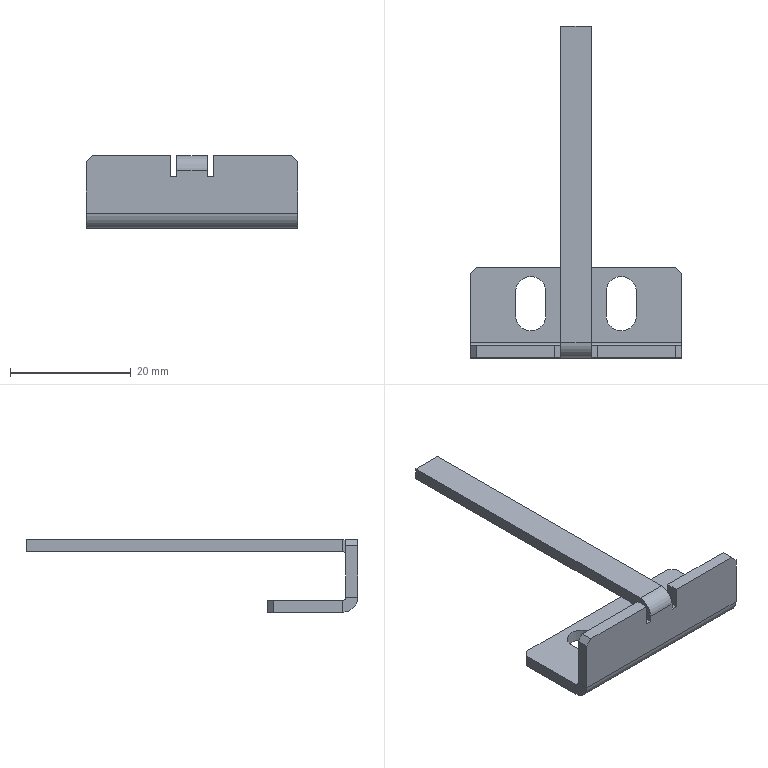Part | SolidWorks | features EdgeFlange 2, Chamfer 1, FlatPattern 1, HoleWzd 1, SMBaseFlange 1, SheetMetal 1 | 1 solid | 42 faces | box 35 x 55 x 12 mm | volume 2052 mm3 | plane 34 | cylinder 8 | commonest cylinder face diameters 5 x6 1 x2
STEP:
#1=CARTESIAN_POINT('',(-16.5,-7.5,10.));
#2=VERTEX_POINT('',#1);
#3=CARTESIAN_POINT('',(-3.5,-7.5,10.));
#4=VERTEX_POINT('',#3);
#5=CARTESIAN_POINT('',(17.5,-7.5,10.));
#6=DIRECTION('',(1.,0.,0.));
#7=VECTOR('',#6,1000.);
#8=LINE('',#5,#7);
#9=EDGE_CURVE('',#2,#4,#8,.T.);
#10=ORIENTED_EDGE('',*,*,#9,.F.);
#11=CARTESIAN_POINT('',(-17.5,-7.5,9.));
#12=VERTEX_POINT('',#11);
#13=CARTESIAN_POINT('',(-13.25,-7.5,13.25));
#14=DIRECTION('',(-0.7071,0.,-0.7071));
#15=VECTOR('',#14,1000.);
#16=LINE('',#13,#15);
#17=EDGE_CURVE('',#2,#12,#16,.T.);
#18=ORIENTED_EDGE('',*,*,#17,.T.);
#19=CARTESIAN_POINT('',(-17.5,-7.5,0.5));
#20=VERTEX_POINT('',#19);
#21=CARTESIAN_POINT('',(-17.5,-7.5,10.));
#22=DIRECTION('',(0.,0.,1.));
#23=VECTOR('',#22,1000.);
#24=LINE('',#21,#23);
#25=EDGE_CURVE('',#20,#12,#24,.T.);
#26=ORIENTED_EDGE('',*,*,#25,.F.);
#27=CARTESIAN_POINT('',(17.5,-7.5,0.5));
#28=VERTEX_POINT('',#27);
#29=CARTESIAN_POINT('',(0.,-7.5,0.5));
#30=DIRECTION('',(1.,0.,0.));
#31=VECTOR('',#30,1000.);
#32=LINE('',#29,#31);
#33=EDGE_CURVE('',#20,#28,#32,.T.);
#34=ORIENTED_EDGE('',*,*,#33,.T.);
#35=CARTESIAN_POINT('',(17.5,-7.5,9.));
#36=VERTEX_POINT('',#35);
#37=CARTESIAN_POINT('',(17.5,-7.5,0.));
#38=DIRECTION('',(0.,0.,-1.));
#39=VECTOR('',#38,1000.);
#40=LINE('',#37,#39);
#41=EDGE_CURVE('',#36,#28,#40,.T.);
#42=ORIENTED_EDGE('',*,*,#41,.F.);
#43=CARTESIAN_POINT('',(16.5,-7.5,10.));
#44=VERTEX_POINT('',#43);
#45=CARTESIAN_POINT('',(13.25,-7.5,13.25));
#46=DIRECTION('',(-0.7071,0.,0.7071));
#47=VECTOR('',#46,1000.);
#48=LINE('',#45,#47);
#49=EDGE_CURVE('',#36,#44,#48,.T.);
#50=ORIENTED_EDGE('',*,*,#49,.T.);
#51=CARTESIAN_POINT('',(3.5,-7.5,10.));
#52=VERTEX_POINT('',#51);
#53=CARTESIAN_POINT('',(17.5,-7.5,10.));
#54=DIRECTION('',(1.,0.,0.));
#55=VECTOR('',#54,1000.);
#56=LINE('',#53,#55);
#57=EDGE_CURVE('',#52,#44,#56,.T.);
#58=ORIENTED_EDGE('',*,*,#57,.F.);
#59=CARTESIAN_POINT('',(3.5,-7.5,6.5));
#60=VERTEX_POINT('',#59);
#61=CARTESIAN_POINT('',(3.5,-7.5,0.));
#62=DIRECTION('',(0.,0.,-1.));
#63=VECTOR('',#62,1000.);
#64=LINE('',#61,#63);
#65=EDGE_CURVE('',#52,#60,#64,.T.);
#66=ORIENTED_EDGE('',*,*,#65,.T.);
#67=CARTESIAN_POINT('',(2.5,-7.5,6.5));
#68=VERTEX_POINT('',#67);
#69=CARTESIAN_POINT('',(0.,-7.5,6.5));
#70=DIRECTION('',(-1.,0.,0.));
#71=VECTOR('',#70,1000.);
#72=LINE('',#69,#71);
#73=EDGE_CURVE('',#60,#68,#72,.T.);
#74=ORIENTED_EDGE('',*,*,#73,.T.);
#75=CARTESIAN_POINT('',(2.5,-7.5,7.5));
#76=VERTEX_POINT('',#75);
#77=CARTESIAN_POINT('',(2.5,-7.5,0.));
#78=DIRECTION('',(0.,0.,1.));
#79=VECTOR('',#78,1000.);
#80=LINE('',#77,#79);
#81=EDGE_CURVE('',#68,#76,#80,.T.);
#82=ORIENTED_EDGE('',*,*,#81,.T.);
#83=CARTESIAN_POINT('',(-2.5,-7.5,7.5));
#84=VERTEX_POINT('',#83);
#85=CARTESIAN_POINT('',(2.5,-7.5,7.5));
#86=DIRECTION('',(-1.,0.,0.));
#87=VECTOR('',#86,1000.);
#88=LINE('',#85,#87);
#89=EDGE_CURVE('',#76,#84,#88,.T.);
#90=ORIENTED_EDGE('',*,*,#89,.T.);
#91=CARTESIAN_POINT('',(-2.5,-7.5,6.5));
#92=VERTEX_POINT('',#91);
#93=CARTESIAN_POINT('',(-2.5,-7.5,0.));
#94=DIRECTION('',(0.,0.,-1.));
#95=VECTOR('',#94,1000.);
#96=LINE('',#93,#95);
#97=EDGE_CURVE('',#84,#92,#96,.T.);
#98=ORIENTED_EDGE('',*,*,#97,.T.);
#99=CARTESIAN_POINT('',(-3.5,-7.5,6.5));
#100=VERTEX_POINT('',#99);
#101=CARTESIAN_POINT('',(0.,-7.5,6.5));
#102=DIRECTION('',(-1.,0.,0.));
#103=VECTOR('',#102,1000.);
#104=LINE('',#101,#103);
#105=EDGE_CURVE('',#92,#100,#104,.T.);
#106=ORIENTED_EDGE('',*,*,#105,.T.);
#107=CARTESIAN_POINT('',(-3.5,-7.5,0.));
#108=DIRECTION('',(0.,0.,1.));
#109=VECTOR('',#108,1000.);
#110=LINE('',#107,#109);
#111=EDGE_CURVE('',#100,#4,#110,.T.);
#112=ORIENTED_EDGE('',*,*,#111,.T.);
#113=EDGE_LOOP('',(#10,#18,#26,#34,#42,#50,#58,#66,#74,#82,#90,#98,#106,#112));
#114=FACE_OUTER_BOUND('',#113,.T.);
#115=CARTESIAN_POINT('',(0.,-7.5,0.));
#116=DIRECTION('',(0.,-1.,0.));
#117=DIRECTION('',(0.,0.,-1.));
#118=AXIS2_PLACEMENT_3D('',#115,#116,#117);
#119=PLANE('',#118);
#120=ADVANCED_FACE('',(#114),#119,.T.);
#121=CARTESIAN_POINT('',(-17.5,-5.5,0.5));
#122=VERTEX_POINT('',#121);
#123=CARTESIAN_POINT('',(-17.5,-5.5,9.));
#124=VERTEX_POINT('',#123);
#125=CARTESIAN_POINT('',(-17.5,-5.5,0.));
#126=DIRECTION('',(0.,0.,1.));
#127=VECTOR('',#126,1000.);
#128=LINE('',#125,#127);
#129=EDGE_CURVE('',#122,#124,#128,.T.);
#130=ORIENTED_EDGE('',*,*,#129,.T.);
#131=CARTESIAN_POINT('',(-16.5,-5.5,10.));
#132=VERTEX_POINT('',#131);
#133=CARTESIAN_POINT('',(-17.5,-5.5,9.));
#134=DIRECTION('',(0.7071,0.,0.7071));
#135=VECTOR('',#134,1000.);
#136=LINE('',#133,#135);
#137=EDGE_CURVE('',#124,#132,#136,.T.);
#138=ORIENTED_EDGE('',*,*,#137,.T.);
#139=CARTESIAN_POINT('',(-3.5,-5.5,10.));
#140=VERTEX_POINT('',#139);
#141=CARTESIAN_POINT('',(0.,-5.5,10.));
#142=DIRECTION('',(1.,0.,0.));
#143=VECTOR('',#142,1000.);
#144=LINE('',#141,#143);
#145=EDGE_CURVE('',#132,#140,#144,.T.);
#146=ORIENTED_EDGE('',*,*,#145,.T.);
#147=CARTESIAN_POINT('',(-3.5,-5.5,6.5));
#148=VERTEX_POINT('',#147);
#149=CARTESIAN_POINT('',(-3.5,-5.5,6.5));
#150=DIRECTION('',(0.,0.,1.));
#151=VECTOR('',#150,1000.);
#152=LINE('',#149,#151);
#153=EDGE_CURVE('',#148,#140,#152,.T.);
#154=ORIENTED_EDGE('',*,*,#153,.F.);
#155=CARTESIAN_POINT('',(-2.5,-5.5,6.5));
#156=VERTEX_POINT('',#155);
#157=CARTESIAN_POINT('',(-2.5,-5.5,6.5));
#158=DIRECTION('',(-1.,0.,0.));
#159=VECTOR('',#158,1000.);
#160=LINE('',#157,#159);
#161=EDGE_CURVE('',#156,#148,#160,.T.);
#162=ORIENTED_EDGE('',*,*,#161,.F.);
#163=CARTESIAN_POINT('',(-2.5,-5.5,7.5));
#164=VERTEX_POINT('',#163);
#165=CARTESIAN_POINT('',(-2.5,-5.5,7.5));
#166=DIRECTION('',(0.,0.,-1.));
#167=VECTOR('',#166,1000.);
#168=LINE('',#165,#167);
#169=EDGE_CURVE('',#164,#156,#168,.T.);
#170=ORIENTED_EDGE('',*,*,#169,.F.);
#171=CARTESIAN_POINT('',(2.5,-5.5,7.5));
#172=VERTEX_POINT('',#171);
#173=CARTESIAN_POINT('',(2.5,-5.5,7.5));
#174=DIRECTION('',(-1.,0.,0.));
#175=VECTOR('',#174,1000.);
#176=LINE('',#173,#175);
#177=EDGE_CURVE('',#172,#164,#176,.T.);
#178=ORIENTED_EDGE('',*,*,#177,.F.);
#179=CARTESIAN_POINT('',(2.5,-5.5,6.5));
#180=VERTEX_POINT('',#179);
#181=CARTESIAN_POINT('',(2.5,-5.5,6.5));
#182=DIRECTION('',(0.,0.,1.));
#183=VECTOR('',#182,1000.);
#184=LINE('',#181,#183);
#185=EDGE_CURVE('',#180,#172,#184,.T.);
#186=ORIENTED_EDGE('',*,*,#185,.F.);
#187=CARTESIAN_POINT('',(3.5,-5.5,6.5));
#188=VERTEX_POINT('',#187);
#189=CARTESIAN_POINT('',(3.5,-5.5,6.5));
#190=DIRECTION('',(-1.,0.,0.));
#191=VECTOR('',#190,1000.);
#192=LINE('',#189,#191);
#193=EDGE_CURVE('',#188,#180,#192,.T.);
#194=ORIENTED_EDGE('',*,*,#193,.F.);
#195=CARTESIAN_POINT('',(3.5,-5.5,10.));
#196=VERTEX_POINT('',#195);
#197=CARTESIAN_POINT('',(3.5,-5.5,10.));
#198=DIRECTION('',(0.,0.,-1.));
#199=VECTOR('',#198,1000.);
#200=LINE('',#197,#199);
#201=EDGE_CURVE('',#196,#188,#200,.T.);
#202=ORIENTED_EDGE('',*,*,#201,.F.);
#203=CARTESIAN_POINT('',(16.5,-5.5,10.));
#204=VERTEX_POINT('',#203);
#205=CARTESIAN_POINT('',(0.,-5.5,10.));
#206=DIRECTION('',(1.,0.,0.));
#207=VECTOR('',#206,1000.);
#208=LINE('',#205,#207);
#209=EDGE_CURVE('',#196,#204,#208,.T.);
#210=ORIENTED_EDGE('',*,*,#209,.T.);
#211=CARTESIAN_POINT('',(17.5,-5.5,9.));
#212=VERTEX_POINT('',#211);
#213=CARTESIAN_POINT('',(16.5,-5.5,10.));
#214=DIRECTION('',(0.7071,0.,-0.7071));
#215=VECTOR('',#214,1000.);
#216=LINE('',#213,#215);
#217=EDGE_CURVE('',#204,#212,#216,.T.);
#218=ORIENTED_EDGE('',*,*,#217,.T.);
#219=CARTESIAN_POINT('',(17.5,-5.5,0.5));
#220=VERTEX_POINT('',#219);
#221=CARTESIAN_POINT('',(17.5,-5.5,0.));
#222=DIRECTION('',(0.,0.,-1.));
#223=VECTOR('',#222,1000.);
#224=LINE('',#221,#223);
#225=EDGE_CURVE('',#212,#220,#224,.T.);
#226=ORIENTED_EDGE('',*,*,#225,.T.);
#227=CARTESIAN_POINT('',(-17.5,-5.5,0.5));
#228=DIRECTION('',(1.,0.,0.));
#229=VECTOR('',#228,1000.);
#230=LINE('',#227,#229);
#231=EDGE_CURVE('',#122,#220,#230,.T.);
#232=ORIENTED_EDGE('',*,*,#231,.F.);
#233=EDGE_LOOP('',(#130,#138,#146,#154,#162,#170,#178,#186,#194,#202,#210,#218,#226,#232));
#234=FACE_OUTER_BOUND('',#233,.T.);
#235=CARTESIAN_POINT('',(0.,-5.5,0.));
#236=DIRECTION('',(0.,-1.,0.));
#237=DIRECTION('',(0.,0.,-1.));
#238=AXIS2_PLACEMENT_3D('',#235,#236,#237);
#239=PLANE('',#238);
#240=ADVANCED_FACE('',(#234),#239,.F.);
#241=ORIENTED_EDGE('',*,*,#57,.T.);
#242=CARTESIAN_POINT('',(16.5,-7.5,10.));
#243=DIRECTION('',(0.,1.,0.));
#244=VECTOR('',#243,1000.);
#245=LINE('',#242,#244);
#246=EDGE_CURVE('',#44,#204,#245,.T.);
#247=ORIENTED_EDGE('',*,*,#246,.T.);
#248=ORIENTED_EDGE('',*,*,#209,.F.);
#249=CARTESIAN_POINT('',(3.5,-5.5,10.));
#250=DIRECTION('',(0.,-1.,0.));
#251=VECTOR('',#250,1000.);
#252=LINE('',#249,#251);
#253=EDGE_CURVE('',#196,#52,#252,.T.);
#254=ORIENTED_EDGE('',*,*,#253,.T.);
#255=EDGE_LOOP('',(#241,#247,#248,#254));
#256=FACE_OUTER_BOUND('',#255,.T.);
#257=CARTESIAN_POINT('',(17.5,-7.5,10.));
#258=DIRECTION('',(0.,0.,1.));
#259=DIRECTION('',(0.,-1.,0.));
#260=AXIS2_PLACEMENT_3D('',#257,#258,#259);
#261=PLANE('',#260);
#262=ADVANCED_FACE('',(#256),#261,.T.);
#263=ORIENTED_EDGE('',*,*,#145,.F.);
#264=CARTESIAN_POINT('',(-16.5,-7.5,10.));
#265=DIRECTION('',(0.,-1.,0.));
#266=VECTOR('',#265,1000.);
#267=LINE('',#264,#266);
#268=EDGE_CURVE('',#132,#2,#267,.T.);
#269=ORIENTED_EDGE('',*,*,#268,.T.);
#270=ORIENTED_EDGE('',*,*,#9,.T.);
#271=CARTESIAN_POINT('',(-3.5,-5.5,10.));
#272=DIRECTION('',(0.,-1.,0.));
#273=VECTOR('',#272,1000.);
#274=LINE('',#271,#273);
#275=EDGE_CURVE('',#140,#4,#274,.T.);
#276=ORIENTED_EDGE('',*,*,#275,.F.);
#277=EDGE_LOOP('',(#263,#269,#270,#276));
#278=FACE_OUTER_BOUND('',#277,.T.);
#279=CARTESIAN_POINT('',(17.5,-7.5,10.));
#280=DIRECTION('',(0.,0.,1.));
#281=DIRECTION('',(0.,-1.,0.));
#282=AXIS2_PLACEMENT_3D('',#279,#280,#281);
#283=PLANE('',#282);
#284=ADVANCED_FACE('',(#278),#283,.T.);
#285=CARTESIAN_POINT('',(17.5,-5.,-2.));
#286=VERTEX_POINT('',#285);
#287=CARTESIAN_POINT('',(17.5,6.5,-2.));
#288=VERTEX_POINT('',#287);
#289=CARTESIAN_POINT('',(17.5,7.5,-2.));
#290=DIRECTION('',(0.,1.,0.));
#291=VECTOR('',#290,1000.);
#292=LINE('',#289,#291);
#293=EDGE_CURVE('',#286,#288,#292,.T.);
#294=ORIENTED_EDGE('',*,*,#293,.T.);
#295=CARTESIAN_POINT('',(17.5,6.5,0.));
#296=VERTEX_POINT('',#295);
#297=CARTESIAN_POINT('',(17.5,6.5,-2.));
#298=DIRECTION('',(0.,0.,1.));
#299=VECTOR('',#298,1000.);
#300=LINE('',#297,#299);
#301=EDGE_CURVE('',#288,#296,#300,.T.);
#302=ORIENTED_EDGE('',*,*,#301,.T.);
#303=CARTESIAN_POINT('',(17.5,-5.,0.));
#304=VERTEX_POINT('',#303);
#305=CARTESIAN_POINT('',(17.5,7.5,0.));
#306=DIRECTION('',(0.,1.,0.));
#307=VECTOR('',#306,1000.);
#308=LINE('',#305,#307);
#309=EDGE_CURVE('',#304,#296,#308,.T.);
#310=ORIENTED_EDGE('',*,*,#309,.F.);
#311=CARTESIAN_POINT('',(17.5,-5.,0.));
#312=DIRECTION('',(0.,0.,-1.));
#313=VECTOR('',#312,1000.);
#314=LINE('',#311,#313);
#315=EDGE_CURVE('',#304,#286,#314,.T.);
#316=ORIENTED_EDGE('',*,*,#315,.T.);
#317=EDGE_LOOP('',(#294,#302,#310,#316));
#318=FACE_OUTER_BOUND('',#317,.T.);
#319=CARTESIAN_POINT('',(17.5,7.5,-2.));
#320=DIRECTION('',(1.,0.,0.));
#321=DIRECTION('',(0.,0.,-1.));
#322=AXIS2_PLACEMENT_3D('',#319,#320,#321);
#323=PLANE('',#322);
#324=ADVANCED_FACE('',(#318),#323,.T.);
#325=CARTESIAN_POINT('',(-10.,-0.5,-2.));
#326=VERTEX_POINT('',#325);
#327=CARTESIAN_POINT('',(-10.,3.5,-2.));
#328=VERTEX_POINT('',#327);
#329=CARTESIAN_POINT('',(-10.,-0.5,-2.));
#330=DIRECTION('',(0.,1.,0.));
#331=VECTOR('',#330,1000.);
#332=LINE('',#329,#331);
#333=EDGE_CURVE('',#326,#328,#332,.T.);
#334=ORIENTED_EDGE('',*,*,#333,.F.);
#335=CARTESIAN_POINT('',(-5.,-0.5,-2.));
#336=VERTEX_POINT('',#335);
#337=CARTESIAN_POINT('',(-7.5,-0.5,-2.));
#338=DIRECTION('',(0.,0.,1.));
#339=DIRECTION('',(1.,0.,0.));
#340=AXIS2_PLACEMENT_3D('',#337,#338,#339);
#341=CIRCLE('',#340,2.5);
#342=EDGE_CURVE('',#326,#336,#341,.T.);
#343=ORIENTED_EDGE('',*,*,#342,.T.);
#344=CARTESIAN_POINT('',(-5.,3.5,-2.));
#345=VERTEX_POINT('',#344);
#346=CARTESIAN_POINT('',(-5.,-0.5,-2.));
#347=DIRECTION('',(0.,1.,0.));
#348=VECTOR('',#347,1000.);
#349=LINE('',#346,#348);
#350=EDGE_CURVE('',#336,#345,#349,.T.);
#351=ORIENTED_EDGE('',*,*,#350,.T.);
#352=CARTESIAN_POINT('',(-7.5,3.5,-2.));
#353=DIRECTION('',(0.,0.,1.));
#354=DIRECTION('',(1.,0.,0.));
#355=AXIS2_PLACEMENT_3D('',#352,#353,#354);
#356=CIRCLE('',#355,2.5);
#357=EDGE_CURVE('',#345,#328,#356,.T.);
#358=ORIENTED_EDGE('',*,*,#357,.T.);
#359=EDGE_LOOP('',(#334,#343,#351,#358));
#360=FACE_BOUND('',#359,.T.);
#361=CARTESIAN_POINT('',(5.,-0.5,-2.));
#362=VERTEX_POINT('',#361);
#363=CARTESIAN_POINT('',(5.,3.5,-2.));
#364=VERTEX_POINT('',#363);
#365=CARTESIAN_POINT('',(5.,-0.5,-2.));
#366=DIRECTION('',(0.,1.,0.));
#367=VECTOR('',#366,1000.);
#368=LINE('',#365,#367);
#369=EDGE_CURVE('',#362,#364,#368,.T.);
#370=ORIENTED_EDGE('',*,*,#369,.F.);
#371=CARTESIAN_POINT('',(10.,-0.5,-2.));
#372=VERTEX_POINT('',#371);
#373=CARTESIAN_POINT('',(7.5,-0.5,-2.));
#374=DIRECTION('',(0.,0.,1.));
#375=DIRECTION('',(1.,0.,0.));
#376=AXIS2_PLACEMENT_3D('',#373,#374,#375);
#377=CIRCLE('',#376,2.5);
#378=EDGE_CURVE('',#362,#372,#377,.T.);
#379=ORIENTED_EDGE('',*,*,#378,.T.);
#380=CARTESIAN_POINT('',(10.,3.5,-2.));
#381=VERTEX_POINT('',#380);
#382=CARTESIAN_POINT('',(10.,-0.5,-2.));
#383=DIRECTION('',(0.,1.,0.));
#384=VECTOR('',#383,1000.);
#385=LINE('',#382,#384);
#386=EDGE_CURVE('',#372,#381,#385,.T.);
#387=ORIENTED_EDGE('',*,*,#386,.T.);
#388=CARTESIAN_POINT('',(7.5,3.5,-2.));
#389=DIRECTION('',(0.,0.,1.));
#390=DIRECTION('',(1.,0.,0.));
#391=AXIS2_PLACEMENT_3D('',#388,#389,#390);
#392=CIRCLE('',#391,2.5);
#393=EDGE_CURVE('',#381,#364,#392,.T.);
#394=ORIENTED_EDGE('',*,*,#393,.T.);
#395=EDGE_LOOP('',(#370,#379,#387,#394));
#396=FACE_BOUND('',#395,.T.);
#397=CARTESIAN_POINT('',(16.5,7.5,-2.));
#398=VERTEX_POINT('',#397);
#399=CARTESIAN_POINT('',(-16.5,7.5,-2.));
#400=VERTEX_POINT('',#399);
#401=CARTESIAN_POINT('',(-17.5,7.5,-2.));
#402=DIRECTION('',(-1.,0.,0.));
#403=VECTOR('',#402,1000.);
#404=LINE('',#401,#403);
#405=EDGE_CURVE('',#398,#400,#404,.T.);
#406=ORIENTED_EDGE('',*,*,#405,.F.);
#407=CARTESIAN_POINT('',(17.5,6.5,-2.));
#408=DIRECTION('',(0.7071,-0.7071,0.));
#409=VECTOR('',#408,1000.);
#410=LINE('',#407,#409);
#411=EDGE_CURVE('',#398,#288,#410,.T.);
#412=ORIENTED_EDGE('',*,*,#411,.T.);
#413=ORIENTED_EDGE('',*,*,#293,.F.);
#414=CARTESIAN_POINT('',(-17.5,-5.,-2.));
#415=VERTEX_POINT('',#414);
#416=CARTESIAN_POINT('',(17.5,-5.,-2.));
#417=DIRECTION('',(-1.,0.,0.));
#418=VECTOR('',#417,1000.);
#419=LINE('',#416,#418);
#420=EDGE_CURVE('',#286,#415,#419,.T.);
#421=ORIENTED_EDGE('',*,*,#420,.T.);
#422=CARTESIAN_POINT('',(-17.5,6.5,-2.));
#423=VERTEX_POINT('',#422);
#424=CARTESIAN_POINT('',(-17.5,7.5,-2.));
#425=DIRECTION('',(0.,-1.,0.));
#426=VECTOR('',#425,1000.);
#427=LINE('',#424,#426);
#428=EDGE_CURVE('',#423,#415,#427,.T.);
#429=ORIENTED_EDGE('',*,*,#428,.F.);
#430=CARTESIAN_POINT('',(-16.5,7.5,-2.));
#431=DIRECTION('',(0.7071,0.7071,0.));
#432=VECTOR('',#431,1000.);
#433=LINE('',#430,#432);
#434=EDGE_CURVE('',#423,#400,#433,.T.);
#435=ORIENTED_EDGE('',*,*,#434,.T.);
#436=EDGE_LOOP('',(#406,#412,#413,#421,#429,#435));
#437=FACE_OUTER_BOUND('',#436,.T.);
#438=CARTESIAN_POINT('',(0.,0.,-2.));
#439=DIRECTION('',(0.,0.,1.));
#440=DIRECTION('',(1.,0.,0.));
#441=AXIS2_PLACEMENT_3D('',#438,#439,#440);
#442=PLANE('',#441);
#443=ADVANCED_FACE('',(#360,#396,#437),#442,.F.);
#444=CARTESIAN_POINT('',(-5.,-0.5,0.));
#445=VERTEX_POINT('',#444);
#446=CARTESIAN_POINT('',(-5.,3.5,0.));
#447=VERTEX_POINT('',#446);
#448=CARTESIAN_POINT('',(-5.,-0.5,0.));
#449=DIRECTION('',(0.,1.,0.));
#450=VECTOR('',#449,1000.);
#451=LINE('',#448,#450);
#452=EDGE_CURVE('',#445,#447,#451,.T.);
#453=ORIENTED_EDGE('',*,*,#452,.F.);
#454=CARTESIAN_POINT('',(-10.,-0.5,0.));
#455=VERTEX_POINT('',#454);
#456=CARTESIAN_POINT('',(-7.5,-0.5,0.));
#457=DIRECTION('',(0.,0.,1.));
#458=DIRECTION('',(1.,0.,0.));
#459=AXIS2_PLACEMENT_3D('',#456,#457,#458);
#460=CIRCLE('',#459,2.5);
#461=EDGE_CURVE('',#455,#445,#460,.T.);
#462=ORIENTED_EDGE('',*,*,#461,.F.);
#463=CARTESIAN_POINT('',(-10.,3.5,0.));
#464=VERTEX_POINT('',#463);
#465=CARTESIAN_POINT('',(-10.,-0.5,0.));
#466=DIRECTION('',(0.,1.,0.));
#467=VECTOR('',#466,1000.);
#468=LINE('',#465,#467);
#469=EDGE_CURVE('',#455,#464,#468,.T.);
#470=ORIENTED_EDGE('',*,*,#469,.T.);
#471=CARTESIAN_POINT('',(-7.5,3.5,0.));
#472=DIRECTION('',(0.,0.,1.));
#473=DIRECTION('',(1.,0.,0.));
#474=AXIS2_PLACEMENT_3D('',#471,#472,#473);
#475=CIRCLE('',#474,2.5);
#476=EDGE_CURVE('',#447,#464,#475,.T.);
#477=ORIENTED_EDGE('',*,*,#476,.F.);
#478=EDGE_LOOP('',(#453,#462,#470,#477));
#479=FACE_BOUND('',#478,.T.);
#480=CARTESIAN_POINT('',(10.,-0.5,0.));
#481=VERTEX_POINT('',#480);
#482=CARTESIAN_POINT('',(10.,3.5,0.));
#483=VERTEX_POINT('',#482);
#484=CARTESIAN_POINT('',(10.,-0.5,0.));
#485=DIRECTION('',(0.,1.,0.));
#486=VECTOR('',#485,1000.);
#487=LINE('',#484,#486);
#488=EDGE_CURVE('',#481,#483,#487,.T.);
#489=ORIENTED_EDGE('',*,*,#488,.F.);
#490=CARTESIAN_POINT('',(5.,-0.5,0.));
#491=VERTEX_POINT('',#490);
#492=CARTESIAN_POINT('',(7.5,-0.5,0.));
#493=DIRECTION('',(0.,0.,1.));
#494=DIRECTION('',(1.,0.,0.));
#495=AXIS2_PLACEMENT_3D('',#492,#493,#494);
#496=CIRCLE('',#495,2.5);
#497=EDGE_CURVE('',#491,#481,#496,.T.);
#498=ORIENTED_EDGE('',*,*,#497,.F.);
#499=CARTESIAN_POINT('',(5.,3.5,0.));
#500=VERTEX_POINT('',#499);
#501=CARTESIAN_POINT('',(5.,-0.5,0.));
#502=DIRECTION('',(0.,1.,0.));
#503=VECTOR('',#502,1000.);
#504=LINE('',#501,#503);
#505=EDGE_CURVE('',#491,#500,#504,.T.);
#506=ORIENTED_EDGE('',*,*,#505,.T.);
#507=CARTESIAN_POINT('',(7.5,3.5,0.));
#508=DIRECTION('',(0.,0.,1.));
#509=DIRECTION('',(1.,0.,0.));
#510=AXIS2_PLACEMENT_3D('',#507,#508,#509);
#511=CIRCLE('',#510,2.5);
#512=EDGE_CURVE('',#483,#500,#511,.T.);
#513=ORIENTED_EDGE('',*,*,#512,.F.);
#514=EDGE_LOOP('',(#489,#498,#506,#513));
#515=FACE_BOUND('',#514,.T.);
#516=ORIENTED_EDGE('',*,*,#309,.T.);
#517=CARTESIAN_POINT('',(16.5,7.5,0.));
#518=VERTEX_POINT('',#517);
#519=CARTESIAN_POINT('',(12.,12.,0.));
#520=DIRECTION('',(-0.7071,0.7071,0.));
#521=VECTOR('',#520,1000.);
#522=LINE('',#519,#521);
#523=EDGE_CURVE('',#296,#518,#522,.T.);
#524=ORIENTED_EDGE('',*,*,#523,.T.);
#525=CARTESIAN_POINT('',(-16.5,7.5,0.));
#526=VERTEX_POINT('',#525);
#527=CARTESIAN_POINT('',(-17.5,7.5,0.));
#528=DIRECTION('',(-1.,0.,0.));
#529=VECTOR('',#528,1000.);
#530=LINE('',#527,#529);
#531=EDGE_CURVE('',#518,#526,#530,.T.);
#532=ORIENTED_EDGE('',*,*,#531,.T.);
#533=CARTESIAN_POINT('',(-17.5,6.5,0.));
#534=VERTEX_POINT('',#533);
#535=CARTESIAN_POINT('',(-12.,12.,0.));
#536=DIRECTION('',(-0.7071,-0.7071,0.));
#537=VECTOR('',#536,1000.);
#538=LINE('',#535,#537);
#539=EDGE_CURVE('',#526,#534,#538,.T.);
#540=ORIENTED_EDGE('',*,*,#539,.T.);
#541=CARTESIAN_POINT('',(-17.5,-5.,0.));
#542=VERTEX_POINT('',#541);
#543=CARTESIAN_POINT('',(-17.5,7.5,0.));
#544=DIRECTION('',(0.,-1.,0.));
#545=VECTOR('',#544,1000.);
#546=LINE('',#543,#545);
#547=EDGE_CURVE('',#534,#542,#546,.T.);
#548=ORIENTED_EDGE('',*,*,#547,.T.);
#549=CARTESIAN_POINT('',(17.5,-5.,0.));
#550=DIRECTION('',(-1.,0.,0.));
#551=VECTOR('',#550,1000.);
#552=LINE('',#549,#551);
#553=EDGE_CURVE('',#304,#542,#552,.T.);
#554=ORIENTED_EDGE('',*,*,#553,.F.);
#555=EDGE_LOOP('',(#516,#524,#532,#540,#548,#554));
#556=FACE_OUTER_BOUND('',#555,.T.);
#557=CARTESIAN_POINT('',(0.,0.,0.));
#558=DIRECTION('',(0.,0.,1.));
#559=DIRECTION('',(1.,0.,0.));
#560=AXIS2_PLACEMENT_3D('',#557,#558,#559);
#561=PLANE('',#560);
#562=ADVANCED_FACE('',(#479,#515,#556),#561,.T.);
#563=ORIENTED_EDGE('',*,*,#547,.F.);
#564=CARTESIAN_POINT('',(-17.5,6.5,-2.));
#565=DIRECTION('',(0.,0.,-1.));
#566=VECTOR('',#565,1000.);
#567=LINE('',#564,#566);
#568=EDGE_CURVE('',#534,#423,#567,.T.);
#569=ORIENTED_EDGE('',*,*,#568,.T.);
#570=ORIENTED_EDGE('',*,*,#428,.T.);
#571=CARTESIAN_POINT('',(-17.5,-5.,0.));
#572=DIRECTION('',(0.,0.,-1.));
#573=VECTOR('',#572,1000.);
#574=LINE('',#571,#573);
#575=EDGE_CURVE('',#542,#415,#574,.T.);
#576=ORIENTED_EDGE('',*,*,#575,.F.);
#577=EDGE_LOOP('',(#563,#569,#570,#576));
#578=FACE_OUTER_BOUND('',#577,.T.);
#579=CARTESIAN_POINT('',(-17.5,7.5,-2.));
#580=DIRECTION('',(-1.,0.,0.));
#581=DIRECTION('',(0.,-1.,0.));
#582=AXIS2_PLACEMENT_3D('',#579,#580,#581);
#583=PLANE('',#582);
#584=ADVANCED_FACE('',(#578),#583,.T.);
#585=ORIENTED_EDGE('',*,*,#531,.F.);
#586=CARTESIAN_POINT('',(16.5,7.5,-2.));
#587=DIRECTION('',(0.,0.,-1.));
#588=VECTOR('',#587,1000.);
#589=LINE('',#586,#588);
#590=EDGE_CURVE('',#518,#398,#589,.T.);
#591=ORIENTED_EDGE('',*,*,#590,.T.);
#592=ORIENTED_EDGE('',*,*,#405,.T.);
#593=CARTESIAN_POINT('',(-16.5,7.5,-2.));
#594=DIRECTION('',(0.,0.,1.));
#595=VECTOR('',#594,1000.);
#596=LINE('',#593,#595);
#597=EDGE_CURVE('',#400,#526,#596,.T.);
#598=ORIENTED_EDGE('',*,*,#597,.T.);
#599=EDGE_LOOP('',(#585,#591,#592,#598));
#600=FACE_OUTER_BOUND('',#599,.T.);
#601=CARTESIAN_POINT('',(-17.5,7.5,-2.));
#602=DIRECTION('',(0.,1.,0.));
#603=DIRECTION('',(0.,0.,1.));
#604=AXIS2_PLACEMENT_3D('',#601,#602,#603);
#605=PLANE('',#604);
#606=ADVANCED_FACE('',(#600),#605,.T.);
#607=CARTESIAN_POINT('',(-17.5,-7.5,0.5));
#608=DIRECTION('',(0.,-1.,0.));
#609=VECTOR('',#608,1000.);
#610=LINE('',#607,#609);
#611=EDGE_CURVE('',#122,#20,#610,.T.);
#612=ORIENTED_EDGE('',*,*,#611,.F.);
#613=CARTESIAN_POINT('',(-17.5,-5.,0.5));
#614=DIRECTION('',(-1.,0.,0.));
#615=DIRECTION('',(0.,0.,-1.));
#616=AXIS2_PLACEMENT_3D('',#613,#614,#615);
#617=CIRCLE('',#616,0.5);
#618=EDGE_CURVE('',#542,#122,#617,.T.);
#619=ORIENTED_EDGE('',*,*,#618,.F.);
#620=ORIENTED_EDGE('',*,*,#575,.T.);
#621=CARTESIAN_POINT('',(-17.5,-5.,0.5));
#622=DIRECTION('',(-1.,0.,0.));
#623=DIRECTION('',(0.,0.,-1.));
#624=AXIS2_PLACEMENT_3D('',#621,#622,#623);
#625=CIRCLE('',#624,2.5);
#626=EDGE_CURVE('',#415,#20,#625,.T.);
#627=ORIENTED_EDGE('',*,*,#626,.T.);
#628=EDGE_LOOP('',(#612,#619,#620,#627));
#629=FACE_OUTER_BOUND('',#628,.T.);
#630=CARTESIAN_POINT('',(-17.5,-5.,0.5));
#631=DIRECTION('',(-1.,0.,0.));
#632=DIRECTION('',(0.,0.,1.));
#633=AXIS2_PLACEMENT_3D('',#630,#631,#632);
#634=PLANE('',#633);
#635=ADVANCED_FACE('',(#629),#634,.T.);
#636=CARTESIAN_POINT('',(17.5,-5.,0.5));
#637=DIRECTION('',(1.,0.,0.));
#638=DIRECTION('',(0.,0.,-1.));
#639=AXIS2_PLACEMENT_3D('',#636,#637,#638);
#640=CIRCLE('',#639,0.5);
#641=EDGE_CURVE('',#220,#304,#640,.T.);
#642=ORIENTED_EDGE('',*,*,#641,.F.);
#643=CARTESIAN_POINT('',(17.5,-5.5,0.5));
#644=DIRECTION('',(0.,-1.,0.));
#645=VECTOR('',#644,1000.);
#646=LINE('',#643,#645);
#647=EDGE_CURVE('',#220,#28,#646,.T.);
#648=ORIENTED_EDGE('',*,*,#647,.T.);
#649=CARTESIAN_POINT('',(17.5,-5.,0.5));
#650=DIRECTION('',(1.,0.,0.));
#651=DIRECTION('',(0.,0.,-1.));
#652=AXIS2_PLACEMENT_3D('',#649,#650,#651);
#653=CIRCLE('',#652,2.5);
#654=EDGE_CURVE('',#28,#286,#653,.T.);
#655=ORIENTED_EDGE('',*,*,#654,.T.);
#656=ORIENTED_EDGE('',*,*,#315,.F.);
#657=EDGE_LOOP('',(#642,#648,#655,#656));
#658=FACE_OUTER_BOUND('',#657,.T.);
#659=CARTESIAN_POINT('',(17.5,-5.,0.5));
#660=DIRECTION('',(-1.,0.,0.));
#661=DIRECTION('',(0.,0.,1.));
#662=AXIS2_PLACEMENT_3D('',#659,#660,#661);
#663=PLANE('',#662);
#664=ADVANCED_FACE('',(#658),#663,.F.);
#665=ORIENTED_EDGE('',*,*,#420,.F.);
#666=ORIENTED_EDGE('',*,*,#654,.F.);
#667=ORIENTED_EDGE('',*,*,#33,.F.);
#668=ORIENTED_EDGE('',*,*,#626,.F.);
#669=EDGE_LOOP('',(#665,#666,#667,#668));
#670=FACE_OUTER_BOUND('',#669,.T.);
#671=CARTESIAN_POINT('',(17.5,-5.,0.5));
#672=DIRECTION('',(1.,0.,0.));
#673=DIRECTION('',(0.,-1.,0.));
#674=AXIS2_PLACEMENT_3D('',#671,#672,#673);
#675=CYLINDRICAL_SURFACE('',#674,2.5);
#676=ADVANCED_FACE('',(#670),#675,.T.);
#677=ORIENTED_EDGE('',*,*,#553,.T.);
#678=ORIENTED_EDGE('',*,*,#618,.T.);
#679=ORIENTED_EDGE('',*,*,#231,.T.);
#680=ORIENTED_EDGE('',*,*,#641,.T.);
#681=EDGE_LOOP('',(#677,#678,#679,#680));
#682=FACE_OUTER_BOUND('',#681,.T.);
#683=CARTESIAN_POINT('',(17.5,-5.,0.5));
#684=DIRECTION('',(1.,0.,0.));
#685=DIRECTION('',(0.,-1.,0.));
#686=AXIS2_PLACEMENT_3D('',#683,#684,#685);
#687=CYLINDRICAL_SURFACE('',#686,0.5);
#688=ADVANCED_FACE('',(#682),#687,.F.);
#689=ORIENTED_EDGE('',*,*,#225,.F.);
#690=CARTESIAN_POINT('',(17.5,-7.5,9.));
#691=DIRECTION('',(0.,-1.,0.));
#692=VECTOR('',#691,1000.);
#693=LINE('',#690,#692);
#694=EDGE_CURVE('',#212,#36,#693,.T.);
#695=ORIENTED_EDGE('',*,*,#694,.T.);
#696=ORIENTED_EDGE('',*,*,#41,.T.);
#697=ORIENTED_EDGE('',*,*,#647,.F.);
#698=EDGE_LOOP('',(#689,#695,#696,#697));
#699=FACE_OUTER_BOUND('',#698,.T.);
#700=CARTESIAN_POINT('',(17.5,-7.5,0.));
#701=DIRECTION('',(1.,0.,0.));
#702=DIRECTION('',(0.,0.,-1.));
#703=AXIS2_PLACEMENT_3D('',#700,#701,#702);
#704=PLANE('',#703);
#705=ADVANCED_FACE('',(#699),#704,.T.);
#706=ORIENTED_EDGE('',*,*,#25,.T.);
#707=CARTESIAN_POINT('',(-17.5,-7.5,9.));
#708=DIRECTION('',(0.,1.,0.));
#709=VECTOR('',#708,1000.);
#710=LINE('',#707,#709);
#711=EDGE_CURVE('',#12,#124,#710,.T.);
#712=ORIENTED_EDGE('',*,*,#711,.T.);
#713=ORIENTED_EDGE('',*,*,#129,.F.);
#714=ORIENTED_EDGE('',*,*,#611,.T.);
#715=EDGE_LOOP('',(#706,#712,#713,#714));
#716=FACE_OUTER_BOUND('',#715,.T.);
#717=CARTESIAN_POINT('',(-17.5,-7.5,10.));
#718=DIRECTION('',(-1.,0.,0.));
#719=DIRECTION('',(0.,0.,1.));
#720=AXIS2_PLACEMENT_3D('',#717,#718,#719);
#721=PLANE('',#720);
#722=ADVANCED_FACE('',(#716),#721,.T.);
#723=ORIENTED_EDGE('',*,*,#65,.F.);
#724=ORIENTED_EDGE('',*,*,#253,.F.);
#725=ORIENTED_EDGE('',*,*,#201,.T.);
#726=CARTESIAN_POINT('',(3.5,-5.5,6.5));
#727=DIRECTION('',(0.,-1.,0.));
#728=VECTOR('',#727,1000.);
#729=LINE('',#726,#728);
#730=EDGE_CURVE('',#188,#60,#729,.T.);
#731=ORIENTED_EDGE('',*,*,#730,.T.);
#732=EDGE_LOOP('',(#723,#724,#725,#731));
#733=FACE_OUTER_BOUND('',#732,.T.);
#734=CARTESIAN_POINT('',(3.5,-5.5,10.));
#735=DIRECTION('',(-1.,0.,0.));
#736=DIRECTION('',(0.,0.,1.));
#737=AXIS2_PLACEMENT_3D('',#734,#735,#736);
#738=PLANE('',#737);
#739=ADVANCED_FACE('',(#733),#738,.T.);
#740=ORIENTED_EDGE('',*,*,#73,.F.);
#741=ORIENTED_EDGE('',*,*,#730,.F.);
#742=ORIENTED_EDGE('',*,*,#193,.T.);
#743=CARTESIAN_POINT('',(2.5,-5.5,6.5));
#744=DIRECTION('',(0.,-1.,0.));
#745=VECTOR('',#744,1000.);
#746=LINE('',#743,#745);
#747=EDGE_CURVE('',#180,#68,#746,.T.);
#748=ORIENTED_EDGE('',*,*,#747,.T.);
#749=EDGE_LOOP('',(#740,#741,#742,#748));
#750=FACE_OUTER_BOUND('',#749,.T.);
#751=CARTESIAN_POINT('',(3.5,-5.5,6.5));
#752=DIRECTION('',(0.,0.,1.));
#753=DIRECTION('',(0.,-1.,0.));
#754=AXIS2_PLACEMENT_3D('',#751,#752,#753);
#755=PLANE('',#754);
#756=ADVANCED_FACE('',(#750),#755,.T.);
#757=ORIENTED_EDGE('',*,*,#81,.F.);
#758=ORIENTED_EDGE('',*,*,#747,.F.);
#759=ORIENTED_EDGE('',*,*,#185,.T.);
#760=CARTESIAN_POINT('',(2.5,-5.5,7.5));
#761=DIRECTION('',(0.,-1.,0.));
#762=VECTOR('',#761,1000.);
#763=LINE('',#760,#762);
#764=EDGE_CURVE('',#172,#76,#763,.T.);
#765=ORIENTED_EDGE('',*,*,#764,.T.);
#766=EDGE_LOOP('',(#757,#758,#759,#765));
#767=FACE_OUTER_BOUND('',#766,.T.);
#768=CARTESIAN_POINT('',(2.5,-5.5,6.5));
#769=DIRECTION('',(1.,0.,0.));
#770=DIRECTION('',(0.,0.,-1.));
#771=AXIS2_PLACEMENT_3D('',#768,#769,#770);
#772=PLANE('',#771);
#773=ADVANCED_FACE('',(#767),#772,.T.);
#774=ORIENTED_EDGE('',*,*,#97,.F.);
#775=CARTESIAN_POINT('',(-2.5,-5.5,7.5));
#776=DIRECTION('',(0.,-1.,0.));
#777=VECTOR('',#776,1000.);
#778=LINE('',#775,#777);
#779=EDGE_CURVE('',#164,#84,#778,.T.);
#780=ORIENTED_EDGE('',*,*,#779,.F.);
#781=ORIENTED_EDGE('',*,*,#169,.T.);
#782=CARTESIAN_POINT('',(-2.5,-5.5,6.5));
#783=DIRECTION('',(0.,-1.,0.));
#784=VECTOR('',#783,1000.);
#785=LINE('',#782,#784);
#786=EDGE_CURVE('',#156,#92,#785,.T.);
#787=ORIENTED_EDGE('',*,*,#786,.T.);
#788=EDGE_LOOP('',(#774,#780,#781,#787));
#789=FACE_OUTER_BOUND('',#788,.T.);
#790=CARTESIAN_POINT('',(-2.5,-5.5,7.5));
#791=DIRECTION('',(-1.,0.,0.));
#792=DIRECTION('',(0.,0.,1.));
#793=AXIS2_PLACEMENT_3D('',#790,#791,#792);
#794=PLANE('',#793);
#795=ADVANCED_FACE('',(#789),#794,.T.);
#796=ORIENTED_EDGE('',*,*,#105,.F.);
#797=ORIENTED_EDGE('',*,*,#786,.F.);
#798=ORIENTED_EDGE('',*,*,#161,.T.);
#799=CARTESIAN_POINT('',(-3.5,-5.5,6.5));
#800=DIRECTION('',(0.,-1.,0.));
#801=VECTOR('',#800,1000.);
#802=LINE('',#799,#801);
#803=EDGE_CURVE('',#148,#100,#802,.T.);
#804=ORIENTED_EDGE('',*,*,#803,.T.);
#805=EDGE_LOOP('',(#796,#797,#798,#804));
#806=FACE_OUTER_BOUND('',#805,.T.);
#807=CARTESIAN_POINT('',(-2.5,-5.5,6.5));
#808=DIRECTION('',(0.,0.,1.));
#809=DIRECTION('',(0.,-1.,0.));
#810=AXIS2_PLACEMENT_3D('',#807,#808,#809);
#811=PLANE('',#810);
#812=ADVANCED_FACE('',(#806),#811,.T.);
#813=ORIENTED_EDGE('',*,*,#111,.F.);
#814=ORIENTED_EDGE('',*,*,#803,.F.);
#815=ORIENTED_EDGE('',*,*,#153,.T.);
#816=ORIENTED_EDGE('',*,*,#275,.T.);
#817=EDGE_LOOP('',(#813,#814,#815,#816));
#818=FACE_OUTER_BOUND('',#817,.T.);
#819=CARTESIAN_POINT('',(-3.5,-5.5,6.5));
#820=DIRECTION('',(1.,0.,0.));
#821=DIRECTION('',(0.,0.,-1.));
#822=AXIS2_PLACEMENT_3D('',#819,#820,#821);
#823=PLANE('',#822);
#824=ADVANCED_FACE('',(#818),#823,.T.);
#825=CARTESIAN_POINT('',(-2.5,-5.,8.));
#826=VERTEX_POINT('',#825);
#827=CARTESIAN_POINT('',(-2.5,-5.,10.));
#828=VERTEX_POINT('',#827);
#829=CARTESIAN_POINT('',(-2.5,-5.,10.));
#830=DIRECTION('',(0.,0.,1.));
#831=VECTOR('',#830,1000.);
#832=LINE('',#829,#831);
#833=EDGE_CURVE('',#826,#828,#832,.T.);
#834=ORIENTED_EDGE('',*,*,#833,.F.);
#835=CARTESIAN_POINT('',(-2.5,-5.,7.5));
#836=DIRECTION('',(-1.,0.,0.));
#837=DIRECTION('',(0.,0.,-1.));
#838=AXIS2_PLACEMENT_3D('',#835,#836,#837);
#839=CIRCLE('',#838,0.5);
#840=EDGE_CURVE('',#164,#826,#839,.T.);
#841=ORIENTED_EDGE('',*,*,#840,.F.);
#842=ORIENTED_EDGE('',*,*,#779,.T.);
#843=CARTESIAN_POINT('',(-2.5,-5.,7.5));
#844=DIRECTION('',(-1.,0.,0.));
#845=DIRECTION('',(0.,0.,-1.));
#846=AXIS2_PLACEMENT_3D('',#843,#844,#845);
#847=CIRCLE('',#846,2.5);
#848=EDGE_CURVE('',#84,#828,#847,.T.);
#849=ORIENTED_EDGE('',*,*,#848,.T.);
#850=EDGE_LOOP('',(#834,#841,#842,#849));
#851=FACE_OUTER_BOUND('',#850,.T.);
#852=CARTESIAN_POINT('',(-2.5,-5.,7.5));
#853=DIRECTION('',(-1.,0.,0.));
#854=DIRECTION('',(0.,0.,1.));
#855=AXIS2_PLACEMENT_3D('',#852,#853,#854);
#856=PLANE('',#855);
#857=ADVANCED_FACE('',(#851),#856,.T.);
#858=CARTESIAN_POINT('',(2.5,-5.,8.));
#859=VERTEX_POINT('',#858);
#860=CARTESIAN_POINT('',(2.5,-5.,7.5));
#861=DIRECTION('',(1.,0.,0.));
#862=DIRECTION('',(0.,0.,-1.));
#863=AXIS2_PLACEMENT_3D('',#860,#861,#862);
#864=CIRCLE('',#863,0.5);
#865=EDGE_CURVE('',#859,#172,#864,.T.);
#866=ORIENTED_EDGE('',*,*,#865,.F.);
#867=CARTESIAN_POINT('',(2.5,-5.,10.));
#868=VERTEX_POINT('',#867);
#869=CARTESIAN_POINT('',(2.5,-5.,8.));
#870=DIRECTION('',(0.,0.,1.));
#871=VECTOR('',#870,1000.);
#872=LINE('',#869,#871);
#873=EDGE_CURVE('',#859,#868,#872,.T.);
#874=ORIENTED_EDGE('',*,*,#873,.T.);
#875=CARTESIAN_POINT('',(2.5,-5.,7.5));
#876=DIRECTION('',(1.,0.,0.));
#877=DIRECTION('',(0.,0.,-1.));
#878=AXIS2_PLACEMENT_3D('',#875,#876,#877);
#879=CIRCLE('',#878,2.5);
#880=EDGE_CURVE('',#868,#76,#879,.T.);
#881=ORIENTED_EDGE('',*,*,#880,.T.);
#882=ORIENTED_EDGE('',*,*,#764,.F.);
#883=EDGE_LOOP('',(#866,#874,#881,#882));
#884=FACE_OUTER_BOUND('',#883,.T.);
#885=CARTESIAN_POINT('',(2.5,-5.,7.5));
#886=DIRECTION('',(-1.,0.,0.));
#887=DIRECTION('',(0.,0.,1.));
#888=AXIS2_PLACEMENT_3D('',#885,#886,#887);
#889=PLANE('',#888);
#890=ADVANCED_FACE('',(#884),#889,.F.);
#891=ORIENTED_EDGE('',*,*,#89,.F.);
#892=ORIENTED_EDGE('',*,*,#880,.F.);
#893=CARTESIAN_POINT('',(0.,-5.,10.));
#894=DIRECTION('',(1.,0.,0.));
#895=VECTOR('',#894,1000.);
#896=LINE('',#893,#895);
#897=EDGE_CURVE('',#828,#868,#896,.T.);
#898=ORIENTED_EDGE('',*,*,#897,.F.);
#899=ORIENTED_EDGE('',*,*,#848,.F.);
#900=EDGE_LOOP('',(#891,#892,#898,#899));
#901=FACE_OUTER_BOUND('',#900,.T.);
#902=CARTESIAN_POINT('',(2.5,-5.,7.5));
#903=DIRECTION('',(1.,0.,0.));
#904=DIRECTION('',(0.,0.,1.));
#905=AXIS2_PLACEMENT_3D('',#902,#903,#904);
#906=CYLINDRICAL_SURFACE('',#905,2.5);
#907=ADVANCED_FACE('',(#901),#906,.T.);
#908=ORIENTED_EDGE('',*,*,#177,.T.);
#909=ORIENTED_EDGE('',*,*,#840,.T.);
#910=CARTESIAN_POINT('',(-2.5,-5.,8.));
#911=DIRECTION('',(1.,0.,0.));
#912=VECTOR('',#911,1000.);
#913=LINE('',#910,#912);
#914=EDGE_CURVE('',#826,#859,#913,.T.);
#915=ORIENTED_EDGE('',*,*,#914,.T.);
#916=ORIENTED_EDGE('',*,*,#865,.T.);
#917=EDGE_LOOP('',(#908,#909,#915,#916));
#918=FACE_OUTER_BOUND('',#917,.T.);
#919=CARTESIAN_POINT('',(2.5,-5.,7.5));
#920=DIRECTION('',(1.,0.,0.));
#921=DIRECTION('',(0.,0.,1.));
#922=AXIS2_PLACEMENT_3D('',#919,#920,#921);
#923=CYLINDRICAL_SURFACE('',#922,0.5);
#924=ADVANCED_FACE('',(#918),#923,.F.);
#925=CARTESIAN_POINT('',(2.5,47.5,10.));
#926=VERTEX_POINT('',#925);
#927=CARTESIAN_POINT('',(2.5,-5.5,10.));
#928=DIRECTION('',(0.,-1.,0.));
#929=VECTOR('',#928,1000.);
#930=LINE('',#927,#929);
#931=EDGE_CURVE('',#926,#868,#930,.T.);
#932=ORIENTED_EDGE('',*,*,#931,.T.);
#933=ORIENTED_EDGE('',*,*,#873,.F.);
#934=CARTESIAN_POINT('',(2.5,47.5,8.));
#935=VERTEX_POINT('',#934);
#936=CARTESIAN_POINT('',(2.5,0.,8.));
#937=DIRECTION('',(0.,-1.,0.));
#938=VECTOR('',#937,1000.);
#939=LINE('',#936,#938);
#940=EDGE_CURVE('',#935,#859,#939,.T.);
#941=ORIENTED_EDGE('',*,*,#940,.F.);
#942=CARTESIAN_POINT('',(2.5,47.5,10.));
#943=DIRECTION('',(0.,0.,-1.));
#944=VECTOR('',#943,1000.);
#945=LINE('',#942,#944);
#946=EDGE_CURVE('',#926,#935,#945,.T.);
#947=ORIENTED_EDGE('',*,*,#946,.F.);
#948=EDGE_LOOP('',(#932,#933,#941,#947));
#949=FACE_OUTER_BOUND('',#948,.T.);
#950=CARTESIAN_POINT('',(2.5,-5.5,10.));
#951=DIRECTION('',(1.,0.,0.));
#952=DIRECTION('',(0.,0.,-1.));
#953=AXIS2_PLACEMENT_3D('',#950,#951,#952);
#954=PLANE('',#953);
#955=ADVANCED_FACE('',(#949),#954,.T.);
#956=CARTESIAN_POINT('',(-2.5,47.5,8.));
#957=VERTEX_POINT('',#956);
#958=CARTESIAN_POINT('',(-2.5,0.,8.));
#959=DIRECTION('',(0.,1.,0.));
#960=VECTOR('',#959,1000.);
#961=LINE('',#958,#960);
#962=EDGE_CURVE('',#826,#957,#961,.T.);
#963=ORIENTED_EDGE('',*,*,#962,.F.);
#964=ORIENTED_EDGE('',*,*,#833,.T.);
#965=CARTESIAN_POINT('',(-2.5,47.5,10.));
#966=VERTEX_POINT('',#965);
#967=CARTESIAN_POINT('',(-2.5,47.5,10.));
#968=DIRECTION('',(0.,1.,0.));
#969=VECTOR('',#968,1000.);
#970=LINE('',#967,#969);
#971=EDGE_CURVE('',#828,#966,#970,.T.);
#972=ORIENTED_EDGE('',*,*,#971,.T.);
#973=CARTESIAN_POINT('',(-2.5,47.5,10.));
#974=DIRECTION('',(0.,0.,-1.));
#975=VECTOR('',#974,1000.);
#976=LINE('',#973,#975);
#977=EDGE_CURVE('',#966,#957,#976,.T.);
#978=ORIENTED_EDGE('',*,*,#977,.T.);
#979=EDGE_LOOP('',(#963,#964,#972,#978));
#980=FACE_OUTER_BOUND('',#979,.T.);
#981=CARTESIAN_POINT('',(-2.5,47.5,10.));
#982=DIRECTION('',(-1.,0.,0.));
#983=DIRECTION('',(0.,0.,1.));
#984=AXIS2_PLACEMENT_3D('',#981,#982,#983);
#985=PLANE('',#984);
#986=ADVANCED_FACE('',(#980),#985,.T.);
#987=ORIENTED_EDGE('',*,*,#971,.F.);
#988=ORIENTED_EDGE('',*,*,#897,.T.);
#989=ORIENTED_EDGE('',*,*,#931,.F.);
#990=CARTESIAN_POINT('',(2.5,47.5,10.));
#991=DIRECTION('',(1.,0.,0.));
#992=VECTOR('',#991,1000.);
#993=LINE('',#990,#992);
#994=EDGE_CURVE('',#966,#926,#993,.T.);
#995=ORIENTED_EDGE('',*,*,#994,.F.);
#996=EDGE_LOOP('',(#987,#988,#989,#995));
#997=FACE_OUTER_BOUND('',#996,.T.);
#998=CARTESIAN_POINT('',(0.,0.,10.));
#999=DIRECTION('',(0.,0.,1.));
#1000=DIRECTION('',(0.,-1.,0.));
#1001=AXIS2_PLACEMENT_3D('',#998,#999,#1000);
#1002=PLANE('',#1001);
#1003=ADVANCED_FACE('',(#997),#1002,.T.);
#1004=ORIENTED_EDGE('',*,*,#914,.F.);
#1005=ORIENTED_EDGE('',*,*,#962,.T.);
#1006=CARTESIAN_POINT('',(0.,47.5,8.));
#1007=DIRECTION('',(1.,0.,0.));
#1008=VECTOR('',#1007,1000.);
#1009=LINE('',#1006,#1008);
#1010=EDGE_CURVE('',#957,#935,#1009,.T.);
#1011=ORIENTED_EDGE('',*,*,#1010,.T.);
#1012=ORIENTED_EDGE('',*,*,#940,.T.);
#1013=EDGE_LOOP('',(#1004,#1005,#1011,#1012));
#1014=FACE_OUTER_BOUND('',#1013,.T.);
#1015=CARTESIAN_POINT('',(0.,0.,8.));
#1016=DIRECTION('',(0.,0.,1.));
#1017=DIRECTION('',(0.,-1.,0.));
#1018=AXIS2_PLACEMENT_3D('',#1015,#1016,#1017);
#1019=PLANE('',#1018);
#1020=ADVANCED_FACE('',(#1014),#1019,.F.);
#1021=ORIENTED_EDGE('',*,*,#1010,.F.);
#1022=ORIENTED_EDGE('',*,*,#977,.F.);
#1023=ORIENTED_EDGE('',*,*,#994,.T.);
#1024=ORIENTED_EDGE('',*,*,#946,.T.);
#1025=EDGE_LOOP('',(#1021,#1022,#1023,#1024));
#1026=FACE_OUTER_BOUND('',#1025,.T.);
#1027=CARTESIAN_POINT('',(2.5,47.5,10.));
#1028=DIRECTION('',(0.,1.,0.));
#1029=DIRECTION('',(0.,0.,1.));
#1030=AXIS2_PLACEMENT_3D('',#1027,#1028,#1029);
#1031=PLANE('',#1030);
#1032=ADVANCED_FACE('',(#1026),#1031,.T.);
#1033=ORIENTED_EDGE('',*,*,#393,.F.);
#1034=CARTESIAN_POINT('',(10.,3.5,-2.));
#1035=DIRECTION('',(0.,0.,-1.));
#1036=VECTOR('',#1035,1000.);
#1037=LINE('',#1034,#1036);
#1038=EDGE_CURVE('',#483,#381,#1037,.T.);
#1039=ORIENTED_EDGE('',*,*,#1038,.F.);
#1040=ORIENTED_EDGE('',*,*,#512,.T.);
#1041=CARTESIAN_POINT('',(5.,3.5,0.));
#1042=DIRECTION('',(0.,0.,1.));
#1043=VECTOR('',#1042,1000.);
#1044=LINE('',#1041,#1043);
#1045=EDGE_CURVE('',#364,#500,#1044,.T.);
#1046=ORIENTED_EDGE('',*,*,#1045,.F.);
#1047=EDGE_LOOP('',(#1033,#1039,#1040,#1046));
#1048=FACE_OUTER_BOUND('',#1047,.T.);
#1049=CARTESIAN_POINT('',(7.5,3.5,0.));
#1050=DIRECTION('',(0.,0.,1.));
#1051=DIRECTION('',(1.,0.,0.));
#1052=AXIS2_PLACEMENT_3D('',#1049,#1050,#1051);
#1053=CYLINDRICAL_SURFACE('',#1052,2.5);
#1054=ADVANCED_FACE('',(#1048),#1053,.F.);
#1055=ORIENTED_EDGE('',*,*,#497,.T.);
#1056=CARTESIAN_POINT('',(10.,-0.5,-2.));
#1057=DIRECTION('',(0.,0.,-1.));
#1058=VECTOR('',#1057,1000.);
#1059=LINE('',#1056,#1058);
#1060=EDGE_CURVE('',#481,#372,#1059,.T.);
#1061=ORIENTED_EDGE('',*,*,#1060,.T.);
#1062=ORIENTED_EDGE('',*,*,#378,.F.);
#1063=CARTESIAN_POINT('',(5.,-0.5,0.));
#1064=DIRECTION('',(0.,0.,-1.));
#1065=VECTOR('',#1064,1000.);
#1066=LINE('',#1063,#1065);
#1067=EDGE_CURVE('',#491,#362,#1066,.T.);
#1068=ORIENTED_EDGE('',*,*,#1067,.F.);
#1069=EDGE_LOOP('',(#1055,#1061,#1062,#1068));
#1070=FACE_OUTER_BOUND('',#1069,.T.);
#1071=CARTESIAN_POINT('',(7.5,-0.5,0.));
#1072=DIRECTION('',(0.,0.,1.));
#1073=DIRECTION('',(1.,0.,0.));
#1074=AXIS2_PLACEMENT_3D('',#1071,#1072,#1073);
#1075=CYLINDRICAL_SURFACE('',#1074,2.5);
#1076=ADVANCED_FACE('',(#1070),#1075,.F.);
#1077=ORIENTED_EDGE('',*,*,#1045,.T.);
#1078=ORIENTED_EDGE('',*,*,#505,.F.);
#1079=ORIENTED_EDGE('',*,*,#1067,.T.);
#1080=ORIENTED_EDGE('',*,*,#369,.T.);
#1081=EDGE_LOOP('',(#1077,#1078,#1079,#1080));
#1082=FACE_OUTER_BOUND('',#1081,.T.);
#1083=CARTESIAN_POINT('',(5.,-0.5,0.));
#1084=DIRECTION('',(-1.,0.,0.));
#1085=DIRECTION('',(0.,0.,1.));
#1086=AXIS2_PLACEMENT_3D('',#1083,#1084,#1085);
#1087=PLANE('',#1086);
#1088=ADVANCED_FACE('',(#1082),#1087,.F.);
#1089=ORIENTED_EDGE('',*,*,#1038,.T.);
#1090=ORIENTED_EDGE('',*,*,#386,.F.);
#1091=ORIENTED_EDGE('',*,*,#1060,.F.);
#1092=ORIENTED_EDGE('',*,*,#488,.T.);
#1093=EDGE_LOOP('',(#1089,#1090,#1091,#1092));
#1094=FACE_OUTER_BOUND('',#1093,.T.);
#1095=CARTESIAN_POINT('',(10.,-0.5,-2.));
#1096=DIRECTION('',(1.,0.,0.));
#1097=DIRECTION('',(0.,0.,-1.));
#1098=AXIS2_PLACEMENT_3D('',#1095,#1096,#1097);
#1099=PLANE('',#1098);
#1100=ADVANCED_FACE('',(#1094),#1099,.F.);
#1101=ORIENTED_EDGE('',*,*,#357,.F.);
#1102=CARTESIAN_POINT('',(-5.,3.5,-2.));
#1103=DIRECTION('',(0.,0.,-1.));
#1104=VECTOR('',#1103,1000.);
#1105=LINE('',#1102,#1104);
#1106=EDGE_CURVE('',#447,#345,#1105,.T.);
#1107=ORIENTED_EDGE('',*,*,#1106,.F.);
#1108=ORIENTED_EDGE('',*,*,#476,.T.);
#1109=CARTESIAN_POINT('',(-10.,3.5,0.));
#1110=DIRECTION('',(0.,0.,1.));
#1111=VECTOR('',#1110,1000.);
#1112=LINE('',#1109,#1111);
#1113=EDGE_CURVE('',#328,#464,#1112,.T.);
#1114=ORIENTED_EDGE('',*,*,#1113,.F.);
#1115=EDGE_LOOP('',(#1101,#1107,#1108,#1114));
#1116=FACE_OUTER_BOUND('',#1115,.T.);
#1117=CARTESIAN_POINT('',(-7.5,3.5,0.));
#1118=DIRECTION('',(0.,0.,1.));
#1119=DIRECTION('',(1.,0.,0.));
#1120=AXIS2_PLACEMENT_3D('',#1117,#1118,#1119);
#1121=CYLINDRICAL_SURFACE('',#1120,2.5);
#1122=ADVANCED_FACE('',(#1116),#1121,.F.);
#1123=ORIENTED_EDGE('',*,*,#461,.T.);
#1124=CARTESIAN_POINT('',(-5.,-0.5,-2.));
#1125=DIRECTION('',(0.,0.,-1.));
#1126=VECTOR('',#1125,1000.);
#1127=LINE('',#1124,#1126);
#1128=EDGE_CURVE('',#445,#336,#1127,.T.);
#1129=ORIENTED_EDGE('',*,*,#1128,.T.);
#1130=ORIENTED_EDGE('',*,*,#342,.F.);
#1131=CARTESIAN_POINT('',(-10.,-0.5,0.));
#1132=DIRECTION('',(0.,0.,-1.));
#1133=VECTOR('',#1132,1000.);
#1134=LINE('',#1131,#1133);
#1135=EDGE_CURVE('',#455,#326,#1134,.T.);
#1136=ORIENTED_EDGE('',*,*,#1135,.F.);
#1137=EDGE_LOOP('',(#1123,#1129,#1130,#1136));
#1138=FACE_OUTER_BOUND('',#1137,.T.);
#1139=CARTESIAN_POINT('',(-7.5,-0.5,0.));
#1140=DIRECTION('',(0.,0.,1.));
#1141=DIRECTION('',(1.,0.,0.));
#1142=AXIS2_PLACEMENT_3D('',#1139,#1140,#1141);
#1143=CYLINDRICAL_SURFACE('',#1142,2.5);
#1144=ADVANCED_FACE('',(#1138),#1143,.F.);
#1145=ORIENTED_EDGE('',*,*,#1113,.T.);
#1146=ORIENTED_EDGE('',*,*,#469,.F.);
#1147=ORIENTED_EDGE('',*,*,#1135,.T.);
#1148=ORIENTED_EDGE('',*,*,#333,.T.);
#1149=EDGE_LOOP('',(#1145,#1146,#1147,#1148));
#1150=FACE_OUTER_BOUND('',#1149,.T.);
#1151=CARTESIAN_POINT('',(-10.,-0.5,0.));
#1152=DIRECTION('',(-1.,0.,0.));
#1153=DIRECTION('',(0.,0.,1.));
#1154=AXIS2_PLACEMENT_3D('',#1151,#1152,#1153);
#1155=PLANE('',#1154);
#1156=ADVANCED_FACE('',(#1150),#1155,.F.);
#1157=ORIENTED_EDGE('',*,*,#1106,.T.);
#1158=ORIENTED_EDGE('',*,*,#350,.F.);
#1159=ORIENTED_EDGE('',*,*,#1128,.F.);
#1160=ORIENTED_EDGE('',*,*,#452,.T.);
#1161=EDGE_LOOP('',(#1157,#1158,#1159,#1160));
#1162=FACE_OUTER_BOUND('',#1161,.T.);
#1163=CARTESIAN_POINT('',(-5.,-0.5,-2.));
#1164=DIRECTION('',(1.,0.,0.));
#1165=DIRECTION('',(0.,0.,-1.));
#1166=AXIS2_PLACEMENT_3D('',#1163,#1164,#1165);
#1167=PLANE('',#1166);
#1168=ADVANCED_FACE('',(#1162),#1167,.F.);
#1169=ORIENTED_EDGE('',*,*,#17,.F.);
#1170=ORIENTED_EDGE('',*,*,#268,.F.);
#1171=ORIENTED_EDGE('',*,*,#137,.F.);
#1172=ORIENTED_EDGE('',*,*,#711,.F.);
#1173=EDGE_LOOP('',(#1169,#1170,#1171,#1172));
#1174=FACE_OUTER_BOUND('',#1173,.T.);
#1175=CARTESIAN_POINT('',(-17.5,-7.5,9.));
#1176=DIRECTION('',(0.7071,0.,-0.7071));
#1177=DIRECTION('',(0.,1.,0.));
#1178=AXIS2_PLACEMENT_3D('',#1175,#1176,#1177);
#1179=PLANE('',#1178);
#1180=ADVANCED_FACE('',(#1174),#1179,.F.);
#1181=ORIENTED_EDGE('',*,*,#49,.F.);
#1182=ORIENTED_EDGE('',*,*,#694,.F.);
#1183=ORIENTED_EDGE('',*,*,#217,.F.);
#1184=ORIENTED_EDGE('',*,*,#246,.F.);
#1185=EDGE_LOOP('',(#1181,#1182,#1183,#1184));
#1186=FACE_OUTER_BOUND('',#1185,.T.);
#1187=CARTESIAN_POINT('',(16.5,-7.5,10.));
#1188=DIRECTION('',(-0.7071,0.,-0.7071));
#1189=DIRECTION('',(0.,1.,0.));
#1190=AXIS2_PLACEMENT_3D('',#1187,#1188,#1189);
#1191=PLANE('',#1190);
#1192=ADVANCED_FACE('',(#1186),#1191,.F.);
#1193=ORIENTED_EDGE('',*,*,#411,.F.);
#1194=ORIENTED_EDGE('',*,*,#590,.F.);
#1195=ORIENTED_EDGE('',*,*,#523,.F.);
#1196=ORIENTED_EDGE('',*,*,#301,.F.);
#1197=EDGE_LOOP('',(#1193,#1194,#1195,#1196));
#1198=FACE_OUTER_BOUND('',#1197,.T.);
#1199=CARTESIAN_POINT('',(17.5,6.5,-2.));
#1200=DIRECTION('',(-0.7071,-0.7071,0.));
#1201=DIRECTION('',(0.,0.,1.));
#1202=AXIS2_PLACEMENT_3D('',#1199,#1200,#1201);
#1203=PLANE('',#1202);
#1204=ADVANCED_FACE('',(#1198),#1203,.F.);
#1205=ORIENTED_EDGE('',*,*,#434,.F.);
#1206=ORIENTED_EDGE('',*,*,#568,.F.);
#1207=ORIENTED_EDGE('',*,*,#539,.F.);
#1208=ORIENTED_EDGE('',*,*,#597,.F.);
#1209=EDGE_LOOP('',(#1205,#1206,#1207,#1208));
#1210=FACE_OUTER_BOUND('',#1209,.T.);
#1211=CARTESIAN_POINT('',(-16.5,7.5,-2.));
#1212=DIRECTION('',(0.7071,-0.7071,0.));
#1213=DIRECTION('',(0.,0.,1.));
#1214=AXIS2_PLACEMENT_3D('',#1211,#1212,#1213);
#1215=PLANE('',#1214);
#1216=ADVANCED_FACE('',(#1210),#1215,.F.);
#1217=CLOSED_SHELL('',(#120,#240,#262,#284,#324,#443,#562,#584,#606,#635,#664,#676,#688,#705,#722,#739,#756,#773,#795,#812,#824,#857,#890,#907,#924,#955,#986,#1003,#1020,#1032,#1054,#1076,#1088,#1100,#1122,#1144,#1156,#1168,#1180,#1192,#1204,#1216));
#1218=MANIFOLD_SOLID_BREP('',#1217);
#1219=CARTESIAN_POINT('',(0.,0.,0.));
#1220=DIRECTION('',(0.,0.,1.));
#1221=DIRECTION('',(1.,0.,0.));
#1222=AXIS2_PLACEMENT_3D('',#1219,#1220,#1221);
#1223=(LENGTH_UNIT()NAMED_UNIT(*)SI_UNIT(.MILLI.,.METRE.));
#1224=UNCERTAINTY_MEASURE_WITH_UNIT(LENGTH_MEASURE(0.00001),#1223,'','');
#1225=(NAMED_UNIT(*)PLANE_ANGLE_UNIT()SI_UNIT($,.RADIAN.));
#1226=(NAMED_UNIT(*)SI_UNIT($,.STERADIAN.)SOLID_ANGLE_UNIT());
#1227=(GEOMETRIC_REPRESENTATION_CONTEXT(3)GLOBAL_UNCERTAINTY_ASSIGNED_CONTEXT((#1224))GLOBAL_UNIT_ASSIGNED_CONTEXT((#1223,#1225,#1226))REPRESENTATION_CONTEXT('',''));
#1228=ADVANCED_BREP_SHAPE_REPRESENTATION('',(#1218,#1222),#1227);